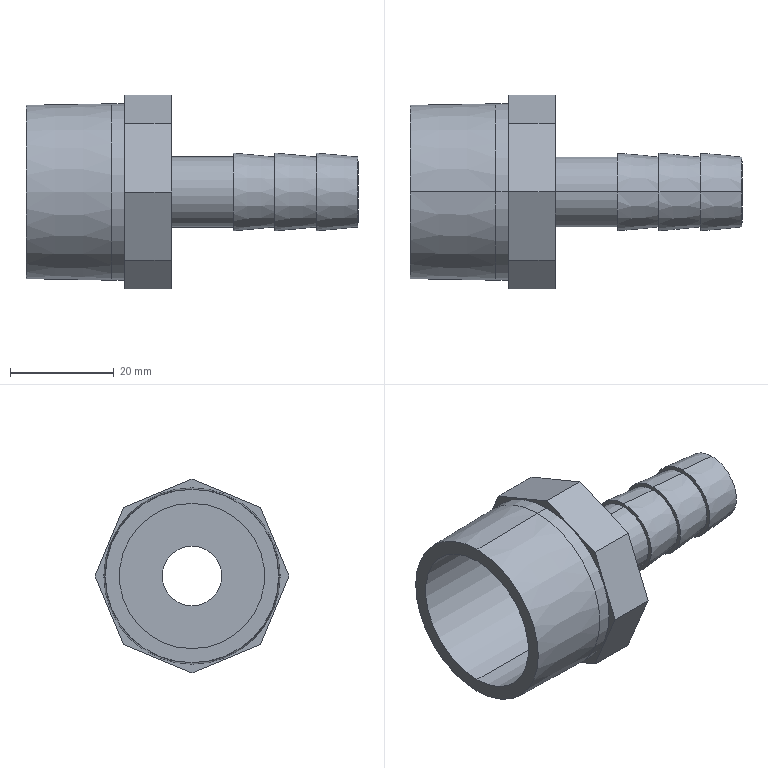Part | SolidWorks | features ICE 1, Revolution 1 | 1 solid | 32 faces | box 64 x 37.343 x 37.343 mm | volume 11465 mm3 | plane 16 | cone 8 | cylinder 8 | commonest cylinder face diameters 11.5 x2 13.5 x2 28 x2 34 x2
STEP:
#1=CARTESIAN_POINT('',(64.,0.,6.75));
#2=VERTEX_POINT('',#1);
#3=CARTESIAN_POINT('',(64.,0.,-6.75));
#4=VERTEX_POINT('',#3);
#5=CARTESIAN_POINT('',(64.,0.,0.));
#6=DIRECTION('',(-1.,0.,0.));
#7=DIRECTION('',(0.,0.,1.));
#8=AXIS2_PLACEMENT_3D('',#5,#6,#7);
#9=CIRCLE('',#8,6.75);
#10=EDGE_CURVE('',#2,#4,#9,.T.);
#11=ORIENTED_EDGE('',*,*,#10,.T.);
#12=CARTESIAN_POINT('',(56.,0.,-7.5));
#13=VERTEX_POINT('',#12);
#14=CARTESIAN_POINT('',(64.,0.,-6.75));
#15=DIRECTION('',(-0.9956,0.,-0.09334));
#16=VECTOR('',#15,1000.);
#17=LINE('',#14,#16);
#18=EDGE_CURVE('',#4,#13,#17,.T.);
#19=ORIENTED_EDGE('',*,*,#18,.T.);
#20=CARTESIAN_POINT('',(56.,0.,7.5));
#21=VERTEX_POINT('',#20);
#22=CARTESIAN_POINT('',(56.,0.,0.));
#23=DIRECTION('',(-1.,0.,0.));
#24=DIRECTION('',(0.,0.,1.));
#25=AXIS2_PLACEMENT_3D('',#22,#23,#24);
#26=CIRCLE('',#25,7.5);
#27=EDGE_CURVE('',#21,#13,#26,.T.);
#28=ORIENTED_EDGE('',*,*,#27,.F.);
#29=CARTESIAN_POINT('',(64.,0.,6.75));
#30=DIRECTION('',(-0.9956,0.,0.09334));
#31=VECTOR('',#30,1000.);
#32=LINE('',#29,#31);
#33=EDGE_CURVE('',#2,#21,#32,.T.);
#34=ORIENTED_EDGE('',*,*,#33,.F.);
#35=EDGE_LOOP('',(#11,#19,#28,#34));
#36=FACE_OUTER_BOUND('',#35,.T.);
#37=CARTESIAN_POINT('',(64.,0.,0.));
#38=DIRECTION('',(-1.,0.,0.));
#39=DIRECTION('',(0.,0.,1.));
#40=AXIS2_PLACEMENT_3D('',#37,#38,#39);
#41=CONICAL_SURFACE('',#40,6.75,0.09348);
#42=ADVANCED_FACE('',(#36),#41,.T.);
#43=CARTESIAN_POINT('',(64.,0.,-5.75));
#44=VERTEX_POINT('',#43);
#45=CARTESIAN_POINT('',(64.,0.,5.75));
#46=VERTEX_POINT('',#45);
#47=CARTESIAN_POINT('',(64.,0.,0.));
#48=DIRECTION('',(-1.,0.,0.));
#49=DIRECTION('',(0.,0.,1.));
#50=AXIS2_PLACEMENT_3D('',#47,#48,#49);
#51=CIRCLE('',#50,5.75);
#52=EDGE_CURVE('',#44,#46,#51,.T.);
#53=ORIENTED_EDGE('',*,*,#52,.F.);
#54=CARTESIAN_POINT('',(26.,0.,-5.75));
#55=VERTEX_POINT('',#54);
#56=CARTESIAN_POINT('',(0.,0.,-5.75));
#57=DIRECTION('',(-1.,0.,0.));
#58=VECTOR('',#57,1000.);
#59=LINE('',#56,#58);
#60=EDGE_CURVE('',#44,#55,#59,.T.);
#61=ORIENTED_EDGE('',*,*,#60,.T.);
#62=CARTESIAN_POINT('',(26.,0.,5.75));
#63=VERTEX_POINT('',#62);
#64=CARTESIAN_POINT('',(26.,0.,0.));
#65=DIRECTION('',(-1.,0.,0.));
#66=DIRECTION('',(0.,0.,1.));
#67=AXIS2_PLACEMENT_3D('',#64,#65,#66);
#68=CIRCLE('',#67,5.75);
#69=EDGE_CURVE('',#55,#63,#68,.T.);
#70=ORIENTED_EDGE('',*,*,#69,.T.);
#71=CARTESIAN_POINT('',(0.,0.,5.75));
#72=DIRECTION('',(-1.,0.,0.));
#73=VECTOR('',#72,1000.);
#74=LINE('',#71,#73);
#75=EDGE_CURVE('',#46,#63,#74,.T.);
#76=ORIENTED_EDGE('',*,*,#75,.F.);
#77=EDGE_LOOP('',(#53,#61,#70,#76));
#78=FACE_OUTER_BOUND('',#77,.T.);
#79=CARTESIAN_POINT('',(0.,0.,0.));
#80=DIRECTION('',(-1.,0.,0.));
#81=DIRECTION('',(0.,0.,1.));
#82=AXIS2_PLACEMENT_3D('',#79,#80,#81);
#83=CYLINDRICAL_SURFACE('',#82,5.75);
#84=ADVANCED_FACE('',(#78),#83,.F.);
#85=CARTESIAN_POINT('',(26.,0.,-14.));
#86=VERTEX_POINT('',#85);
#87=CARTESIAN_POINT('',(26.,0.,14.));
#88=VERTEX_POINT('',#87);
#89=CARTESIAN_POINT('',(26.,0.,0.));
#90=DIRECTION('',(-1.,0.,0.));
#91=DIRECTION('',(0.,0.,1.));
#92=AXIS2_PLACEMENT_3D('',#89,#90,#91);
#93=CIRCLE('',#92,14.);
#94=EDGE_CURVE('',#86,#88,#93,.T.);
#95=ORIENTED_EDGE('',*,*,#94,.F.);
#96=CARTESIAN_POINT('',(0.,0.,-14.));
#97=VERTEX_POINT('',#96);
#98=CARTESIAN_POINT('',(0.,0.,-14.));
#99=DIRECTION('',(-1.,0.,0.));
#100=VECTOR('',#99,1000.);
#101=LINE('',#98,#100);
#102=EDGE_CURVE('',#86,#97,#101,.T.);
#103=ORIENTED_EDGE('',*,*,#102,.T.);
#104=CARTESIAN_POINT('',(0.,0.,14.));
#105=VERTEX_POINT('',#104);
#106=CARTESIAN_POINT('',(0.,0.,0.));
#107=DIRECTION('',(-1.,0.,0.));
#108=DIRECTION('',(0.,0.,1.));
#109=AXIS2_PLACEMENT_3D('',#106,#107,#108);
#110=CIRCLE('',#109,14.);
#111=EDGE_CURVE('',#97,#105,#110,.T.);
#112=ORIENTED_EDGE('',*,*,#111,.T.);
#113=CARTESIAN_POINT('',(0.,0.,14.));
#114=DIRECTION('',(-1.,0.,0.));
#115=VECTOR('',#114,1000.);
#116=LINE('',#113,#115);
#117=EDGE_CURVE('',#88,#105,#116,.T.);
#118=ORIENTED_EDGE('',*,*,#117,.F.);
#119=EDGE_LOOP('',(#95,#103,#112,#118));
#120=FACE_OUTER_BOUND('',#119,.T.);
#121=CARTESIAN_POINT('',(0.,0.,0.));
#122=DIRECTION('',(-1.,0.,0.));
#123=DIRECTION('',(0.,0.,1.));
#124=AXIS2_PLACEMENT_3D('',#121,#122,#123);
#125=CYLINDRICAL_SURFACE('',#124,14.);
#126=ADVANCED_FACE('',(#120),#125,.F.);
#127=CARTESIAN_POINT('',(0.,0.,16.712));
#128=VERTEX_POINT('',#127);
#129=CARTESIAN_POINT('',(0.,0.,-16.712));
#130=VERTEX_POINT('',#129);
#131=CARTESIAN_POINT('',(0.,0.,0.));
#132=DIRECTION('',(-1.,0.,0.));
#133=DIRECTION('',(0.,0.,1.));
#134=AXIS2_PLACEMENT_3D('',#131,#132,#133);
#135=CIRCLE('',#134,16.712);
#136=EDGE_CURVE('',#128,#130,#135,.T.);
#137=ORIENTED_EDGE('',*,*,#136,.F.);
#138=CARTESIAN_POINT('',(16.5,0.,17.));
#139=VERTEX_POINT('',#138);
#140=CARTESIAN_POINT('',(16.5,0.,17.));
#141=DIRECTION('',(0.9998,0.,0.01745));
#142=VECTOR('',#141,1000.);
#143=LINE('',#140,#142);
#144=EDGE_CURVE('',#128,#139,#143,.T.);
#145=ORIENTED_EDGE('',*,*,#144,.T.);
#146=CARTESIAN_POINT('',(16.5,0.,-17.));
#147=VERTEX_POINT('',#146);
#148=CARTESIAN_POINT('',(16.5,0.,0.));
#149=DIRECTION('',(-1.,0.,0.));
#150=DIRECTION('',(0.,0.,1.));
#151=AXIS2_PLACEMENT_3D('',#148,#149,#150);
#152=CIRCLE('',#151,17.);
#153=EDGE_CURVE('',#139,#147,#152,.T.);
#154=ORIENTED_EDGE('',*,*,#153,.T.);
#155=CARTESIAN_POINT('',(16.5,0.,-17.));
#156=DIRECTION('',(0.9998,0.,-0.01745));
#157=VECTOR('',#156,1000.);
#158=LINE('',#155,#157);
#159=EDGE_CURVE('',#130,#147,#158,.T.);
#160=ORIENTED_EDGE('',*,*,#159,.F.);
#161=EDGE_LOOP('',(#137,#145,#154,#160));
#162=FACE_OUTER_BOUND('',#161,.T.);
#163=CARTESIAN_POINT('',(16.5,0.,0.));
#164=DIRECTION('',(1.,0.,0.));
#165=DIRECTION('',(0.,0.,-1.));
#166=AXIS2_PLACEMENT_3D('',#163,#164,#165);
#167=CONICAL_SURFACE('',#166,17.,0.01745);
#168=ADVANCED_FACE('',(#162),#167,.T.);
#169=CARTESIAN_POINT('',(19.,0.,17.));
#170=VERTEX_POINT('',#169);
#171=CARTESIAN_POINT('',(19.,0.,-17.));
#172=VERTEX_POINT('',#171);
#173=CARTESIAN_POINT('',(19.,0.,0.));
#174=DIRECTION('',(-1.,0.,0.));
#175=DIRECTION('',(0.,0.,1.));
#176=AXIS2_PLACEMENT_3D('',#173,#174,#175);
#177=CIRCLE('',#176,17.);
#178=EDGE_CURVE('',#170,#172,#177,.T.);
#179=ORIENTED_EDGE('',*,*,#178,.T.);
#180=CARTESIAN_POINT('',(0.,0.,-17.));
#181=DIRECTION('',(-1.,0.,0.));
#182=VECTOR('',#181,1000.);
#183=LINE('',#180,#182);
#184=EDGE_CURVE('',#172,#147,#183,.T.);
#185=ORIENTED_EDGE('',*,*,#184,.T.);
#186=ORIENTED_EDGE('',*,*,#153,.F.);
#187=CARTESIAN_POINT('',(0.,0.,17.));
#188=DIRECTION('',(-1.,0.,0.));
#189=VECTOR('',#188,1000.);
#190=LINE('',#187,#189);
#191=EDGE_CURVE('',#170,#139,#190,.T.);
#192=ORIENTED_EDGE('',*,*,#191,.F.);
#193=EDGE_LOOP('',(#179,#185,#186,#192));
#194=FACE_OUTER_BOUND('',#193,.T.);
#195=CARTESIAN_POINT('',(0.,0.,0.));
#196=DIRECTION('',(-1.,0.,0.));
#197=DIRECTION('',(0.,0.,1.));
#198=AXIS2_PLACEMENT_3D('',#195,#196,#197);
#199=CYLINDRICAL_SURFACE('',#198,17.);
#200=ADVANCED_FACE('',(#194),#199,.T.);
#201=CARTESIAN_POINT('',(40.,0.,6.75));
#202=VERTEX_POINT('',#201);
#203=CARTESIAN_POINT('',(40.,0.,-6.75));
#204=VERTEX_POINT('',#203);
#205=CARTESIAN_POINT('',(40.,0.,0.));
#206=DIRECTION('',(-1.,0.,0.));
#207=DIRECTION('',(0.,0.,1.));
#208=AXIS2_PLACEMENT_3D('',#205,#206,#207);
#209=CIRCLE('',#208,6.75);
#210=EDGE_CURVE('',#202,#204,#209,.T.);
#211=ORIENTED_EDGE('',*,*,#210,.T.);
#212=CARTESIAN_POINT('',(28.,0.,-6.75));
#213=VERTEX_POINT('',#212);
#214=CARTESIAN_POINT('',(0.,0.,-6.75));
#215=DIRECTION('',(-1.,0.,0.));
#216=VECTOR('',#215,1000.);
#217=LINE('',#214,#216);
#218=EDGE_CURVE('',#204,#213,#217,.T.);
#219=ORIENTED_EDGE('',*,*,#218,.T.);
#220=CARTESIAN_POINT('',(28.,0.,6.75));
#221=VERTEX_POINT('',#220);
#222=CARTESIAN_POINT('',(28.,0.,0.));
#223=DIRECTION('',(-1.,0.,0.));
#224=DIRECTION('',(0.,0.,1.));
#225=AXIS2_PLACEMENT_3D('',#222,#223,#224);
#226=CIRCLE('',#225,6.75);
#227=EDGE_CURVE('',#221,#213,#226,.T.);
#228=ORIENTED_EDGE('',*,*,#227,.F.);
#229=CARTESIAN_POINT('',(0.,0.,6.75));
#230=DIRECTION('',(-1.,0.,0.));
#231=VECTOR('',#230,1000.);
#232=LINE('',#229,#231);
#233=EDGE_CURVE('',#202,#221,#232,.T.);
#234=ORIENTED_EDGE('',*,*,#233,.F.);
#235=EDGE_LOOP('',(#211,#219,#228,#234));
#236=FACE_OUTER_BOUND('',#235,.T.);
#237=CARTESIAN_POINT('',(0.,0.,0.));
#238=DIRECTION('',(-1.,0.,0.));
#239=DIRECTION('',(0.,0.,1.));
#240=AXIS2_PLACEMENT_3D('',#237,#238,#239);
#241=CYLINDRICAL_SURFACE('',#240,6.75);
#242=ADVANCED_FACE('',(#236),#241,.T.);
#243=CARTESIAN_POINT('',(48.,0.,6.75));
#244=VERTEX_POINT('',#243);
#245=CARTESIAN_POINT('',(48.,0.,-6.75));
#246=VERTEX_POINT('',#245);
#247=CARTESIAN_POINT('',(48.,0.,0.));
#248=DIRECTION('',(-1.,0.,0.));
#249=DIRECTION('',(0.,0.,1.));
#250=AXIS2_PLACEMENT_3D('',#247,#248,#249);
#251=CIRCLE('',#250,6.75);
#252=EDGE_CURVE('',#244,#246,#251,.T.);
#253=ORIENTED_EDGE('',*,*,#252,.T.);
#254=CARTESIAN_POINT('',(40.,0.,-7.5));
#255=VERTEX_POINT('',#254);
#256=CARTESIAN_POINT('',(48.,0.,-6.75));
#257=DIRECTION('',(-0.9956,0.,-0.09334));
#258=VECTOR('',#257,1000.);
#259=LINE('',#256,#258);
#260=EDGE_CURVE('',#246,#255,#259,.T.);
#261=ORIENTED_EDGE('',*,*,#260,.T.);
#262=CARTESIAN_POINT('',(40.,0.,7.5));
#263=VERTEX_POINT('',#262);
#264=CARTESIAN_POINT('',(40.,0.,0.));
#265=DIRECTION('',(-1.,0.,0.));
#266=DIRECTION('',(0.,0.,1.));
#267=AXIS2_PLACEMENT_3D('',#264,#265,#266);
#268=CIRCLE('',#267,7.5);
#269=EDGE_CURVE('',#263,#255,#268,.T.);
#270=ORIENTED_EDGE('',*,*,#269,.F.);
#271=CARTESIAN_POINT('',(48.,0.,6.75));
#272=DIRECTION('',(-0.9956,0.,0.09334));
#273=VECTOR('',#272,1000.);
#274=LINE('',#271,#273);
#275=EDGE_CURVE('',#244,#263,#274,.T.);
#276=ORIENTED_EDGE('',*,*,#275,.F.);
#277=EDGE_LOOP('',(#253,#261,#270,#276));
#278=FACE_OUTER_BOUND('',#277,.T.);
#279=CARTESIAN_POINT('',(48.,0.,0.));
#280=DIRECTION('',(-1.,0.,0.));
#281=DIRECTION('',(0.,0.,1.));
#282=AXIS2_PLACEMENT_3D('',#279,#280,#281);
#283=CONICAL_SURFACE('',#282,6.75,0.09348);
#284=ADVANCED_FACE('',(#278),#283,.T.);
#285=CARTESIAN_POINT('',(56.,0.,6.75));
#286=VERTEX_POINT('',#285);
#287=CARTESIAN_POINT('',(56.,0.,-6.75));
#288=VERTEX_POINT('',#287);
#289=CARTESIAN_POINT('',(56.,0.,0.));
#290=DIRECTION('',(-1.,0.,0.));
#291=DIRECTION('',(0.,0.,1.));
#292=AXIS2_PLACEMENT_3D('',#289,#290,#291);
#293=CIRCLE('',#292,6.75);
#294=EDGE_CURVE('',#286,#288,#293,.T.);
#295=ORIENTED_EDGE('',*,*,#294,.T.);
#296=CARTESIAN_POINT('',(48.,0.,-7.5));
#297=VERTEX_POINT('',#296);
#298=CARTESIAN_POINT('',(56.,0.,-6.75));
#299=DIRECTION('',(-0.9956,0.,-0.09334));
#300=VECTOR('',#299,1000.);
#301=LINE('',#298,#300);
#302=EDGE_CURVE('',#288,#297,#301,.T.);
#303=ORIENTED_EDGE('',*,*,#302,.T.);
#304=CARTESIAN_POINT('',(48.,0.,7.5));
#305=VERTEX_POINT('',#304);
#306=CARTESIAN_POINT('',(48.,0.,0.));
#307=DIRECTION('',(-1.,0.,0.));
#308=DIRECTION('',(0.,0.,1.));
#309=AXIS2_PLACEMENT_3D('',#306,#307,#308);
#310=CIRCLE('',#309,7.5);
#311=EDGE_CURVE('',#305,#297,#310,.T.);
#312=ORIENTED_EDGE('',*,*,#311,.F.);
#313=CARTESIAN_POINT('',(56.,0.,6.75));
#314=DIRECTION('',(-0.9956,0.,0.09334));
#315=VECTOR('',#314,1000.);
#316=LINE('',#313,#315);
#317=EDGE_CURVE('',#286,#305,#316,.T.);
#318=ORIENTED_EDGE('',*,*,#317,.F.);
#319=EDGE_LOOP('',(#295,#303,#312,#318));
#320=FACE_OUTER_BOUND('',#319,.T.);
#321=CARTESIAN_POINT('',(56.,0.,0.));
#322=DIRECTION('',(-1.,0.,0.));
#323=DIRECTION('',(0.,0.,1.));
#324=AXIS2_PLACEMENT_3D('',#321,#322,#323);
#325=CONICAL_SURFACE('',#324,6.75,0.09348);
#326=ADVANCED_FACE('',(#320),#325,.T.);
#327=ORIENTED_EDGE('',*,*,#302,.F.);
#328=CARTESIAN_POINT('',(56.,0.,0.));
#329=DIRECTION('',(-1.,0.,0.));
#330=DIRECTION('',(0.,0.,1.));
#331=AXIS2_PLACEMENT_3D('',#328,#329,#330);
#332=CIRCLE('',#331,6.75);
#333=EDGE_CURVE('',#288,#286,#332,.T.);
#334=ORIENTED_EDGE('',*,*,#333,.T.);
#335=ORIENTED_EDGE('',*,*,#317,.T.);
#336=CARTESIAN_POINT('',(48.,0.,0.));
#337=DIRECTION('',(-1.,0.,0.));
#338=DIRECTION('',(0.,0.,1.));
#339=AXIS2_PLACEMENT_3D('',#336,#337,#338);
#340=CIRCLE('',#339,7.5);
#341=EDGE_CURVE('',#297,#305,#340,.T.);
#342=ORIENTED_EDGE('',*,*,#341,.F.);
#343=EDGE_LOOP('',(#327,#334,#335,#342));
#344=FACE_OUTER_BOUND('',#343,.T.);
#345=CARTESIAN_POINT('',(56.,0.,0.));
#346=DIRECTION('',(-1.,0.,0.));
#347=DIRECTION('',(0.,0.,1.));
#348=AXIS2_PLACEMENT_3D('',#345,#346,#347);
#349=CONICAL_SURFACE('',#348,6.75,0.09348);
#350=ADVANCED_FACE('',(#344),#349,.T.);
#351=ORIENTED_EDGE('',*,*,#252,.F.);
#352=CARTESIAN_POINT('',(48.,0.,0.));
#353=DIRECTION('',(-1.,0.,0.));
#354=DIRECTION('',(0.,0.,1.));
#355=AXIS2_PLACEMENT_3D('',#352,#353,#354);
#356=CIRCLE('',#355,6.75);
#357=EDGE_CURVE('',#246,#244,#356,.T.);
#358=ORIENTED_EDGE('',*,*,#357,.F.);
#359=EDGE_LOOP('',(#351,#358));
#360=FACE_BOUND('',#359,.T.);
#361=ORIENTED_EDGE('',*,*,#311,.T.);
#362=ORIENTED_EDGE('',*,*,#341,.T.);
#363=EDGE_LOOP('',(#361,#362));
#364=FACE_OUTER_BOUND('',#363,.T.);
#365=CARTESIAN_POINT('',(48.,7.5,0.));
#366=DIRECTION('',(1.,0.,0.));
#367=DIRECTION('',(0.,0.,-1.));
#368=AXIS2_PLACEMENT_3D('',#365,#366,#367);
#369=PLANE('',#368);
#370=ADVANCED_FACE('',(#360,#364),#369,.F.);
#371=ORIENTED_EDGE('',*,*,#260,.F.);
#372=ORIENTED_EDGE('',*,*,#357,.T.);
#373=ORIENTED_EDGE('',*,*,#275,.T.);
#374=CARTESIAN_POINT('',(40.,0.,0.));
#375=DIRECTION('',(-1.,0.,0.));
#376=DIRECTION('',(0.,0.,1.));
#377=AXIS2_PLACEMENT_3D('',#374,#375,#376);
#378=CIRCLE('',#377,7.5);
#379=EDGE_CURVE('',#255,#263,#378,.T.);
#380=ORIENTED_EDGE('',*,*,#379,.F.);
#381=EDGE_LOOP('',(#371,#372,#373,#380));
#382=FACE_OUTER_BOUND('',#381,.T.);
#383=CARTESIAN_POINT('',(48.,0.,0.));
#384=DIRECTION('',(-1.,0.,0.));
#385=DIRECTION('',(0.,0.,1.));
#386=AXIS2_PLACEMENT_3D('',#383,#384,#385);
#387=CONICAL_SURFACE('',#386,6.75,0.09348);
#388=ADVANCED_FACE('',(#382),#387,.T.);
#389=ORIENTED_EDGE('',*,*,#210,.F.);
#390=CARTESIAN_POINT('',(40.,0.,0.));
#391=DIRECTION('',(-1.,0.,0.));
#392=DIRECTION('',(0.,0.,1.));
#393=AXIS2_PLACEMENT_3D('',#390,#391,#392);
#394=CIRCLE('',#393,6.75);
#395=EDGE_CURVE('',#204,#202,#394,.T.);
#396=ORIENTED_EDGE('',*,*,#395,.F.);
#397=EDGE_LOOP('',(#389,#396));
#398=FACE_BOUND('',#397,.T.);
#399=ORIENTED_EDGE('',*,*,#269,.T.);
#400=ORIENTED_EDGE('',*,*,#379,.T.);
#401=EDGE_LOOP('',(#399,#400));
#402=FACE_OUTER_BOUND('',#401,.T.);
#403=CARTESIAN_POINT('',(40.,7.5,0.));
#404=DIRECTION('',(1.,0.,0.));
#405=DIRECTION('',(0.,0.,-1.));
#406=AXIS2_PLACEMENT_3D('',#403,#404,#405);
#407=PLANE('',#406);
#408=ADVANCED_FACE('',(#398,#402),#407,.F.);
#409=ORIENTED_EDGE('',*,*,#218,.F.);
#410=ORIENTED_EDGE('',*,*,#395,.T.);
#411=ORIENTED_EDGE('',*,*,#233,.T.);
#412=CARTESIAN_POINT('',(28.,0.,0.));
#413=DIRECTION('',(-1.,0.,0.));
#414=DIRECTION('',(0.,0.,1.));
#415=AXIS2_PLACEMENT_3D('',#412,#413,#414);
#416=CIRCLE('',#415,6.75);
#417=EDGE_CURVE('',#213,#221,#416,.T.);
#418=ORIENTED_EDGE('',*,*,#417,.F.);
#419=EDGE_LOOP('',(#409,#410,#411,#418));
#420=FACE_OUTER_BOUND('',#419,.T.);
#421=CARTESIAN_POINT('',(0.,0.,0.));
#422=DIRECTION('',(-1.,0.,0.));
#423=DIRECTION('',(0.,0.,1.));
#424=AXIS2_PLACEMENT_3D('',#421,#422,#423);
#425=CYLINDRICAL_SURFACE('',#424,6.75);
#426=ADVANCED_FACE('',(#420),#425,.T.);
#427=CARTESIAN_POINT('',(28.,-13.203,-13.203));
#428=VERTEX_POINT('',#427);
#429=CARTESIAN_POINT('',(28.,0.,-18.671));
#430=VERTEX_POINT('',#429);
#431=CARTESIAN_POINT('',(28.,-13.203,-13.203));
#432=DIRECTION('',(0.,0.9239,-0.3827));
#433=VECTOR('',#432,1000.);
#434=LINE('',#431,#433);
#435=EDGE_CURVE('',#428,#430,#434,.T.);
#436=ORIENTED_EDGE('',*,*,#435,.T.);
#437=CARTESIAN_POINT('',(28.,13.203,-13.203));
#438=VERTEX_POINT('',#437);
#439=CARTESIAN_POINT('',(28.,0.,-18.671));
#440=DIRECTION('',(0.,0.9239,0.3827));
#441=VECTOR('',#440,1000.);
#442=LINE('',#439,#441);
#443=EDGE_CURVE('',#430,#438,#442,.T.);
#444=ORIENTED_EDGE('',*,*,#443,.T.);
#445=CARTESIAN_POINT('',(28.,18.671,0.));
#446=VERTEX_POINT('',#445);
#447=CARTESIAN_POINT('',(28.,13.203,-13.203));
#448=DIRECTION('',(0.,0.3827,0.9239));
#449=VECTOR('',#448,1000.);
#450=LINE('',#447,#449);
#451=EDGE_CURVE('',#438,#446,#450,.T.);
#452=ORIENTED_EDGE('',*,*,#451,.T.);
#453=CARTESIAN_POINT('',(28.,13.203,13.203));
#454=VERTEX_POINT('',#453);
#455=CARTESIAN_POINT('',(28.,18.671,0.));
#456=DIRECTION('',(0.,-0.3827,0.9239));
#457=VECTOR('',#456,1000.);
#458=LINE('',#455,#457);
#459=EDGE_CURVE('',#446,#454,#458,.T.);
#460=ORIENTED_EDGE('',*,*,#459,.T.);
#461=CARTESIAN_POINT('',(28.,0.,18.671));
#462=VERTEX_POINT('',#461);
#463=CARTESIAN_POINT('',(28.,13.203,13.203));
#464=DIRECTION('',(0.,-0.9239,0.3827));
#465=VECTOR('',#464,1000.);
#466=LINE('',#463,#465);
#467=EDGE_CURVE('',#454,#462,#466,.T.);
#468=ORIENTED_EDGE('',*,*,#467,.T.);
#469=CARTESIAN_POINT('',(28.,-13.203,13.203));
#470=VERTEX_POINT('',#469);
#471=CARTESIAN_POINT('',(28.,0.,18.671));
#472=DIRECTION('',(0.,-0.9239,-0.3827));
#473=VECTOR('',#472,1000.);
#474=LINE('',#471,#473);
#475=EDGE_CURVE('',#462,#470,#474,.T.);
#476=ORIENTED_EDGE('',*,*,#475,.T.);
#477=CARTESIAN_POINT('',(28.,-18.671,0.));
#478=VERTEX_POINT('',#477);
#479=CARTESIAN_POINT('',(28.,-13.203,13.203));
#480=DIRECTION('',(0.,-0.3827,-0.9239));
#481=VECTOR('',#480,1000.);
#482=LINE('',#479,#481);
#483=EDGE_CURVE('',#470,#478,#482,.T.);
#484=ORIENTED_EDGE('',*,*,#483,.T.);
#485=CARTESIAN_POINT('',(28.,-18.671,0.));
#486=DIRECTION('',(0.,0.3827,-0.9239));
#487=VECTOR('',#486,1000.);
#488=LINE('',#485,#487);
#489=EDGE_CURVE('',#478,#428,#488,.T.);
#490=ORIENTED_EDGE('',*,*,#489,.T.);
#491=EDGE_LOOP('',(#436,#444,#452,#460,#468,#476,#484,#490));
#492=FACE_OUTER_BOUND('',#491,.T.);
#493=ORIENTED_EDGE('',*,*,#227,.T.);
#494=ORIENTED_EDGE('',*,*,#417,.T.);
#495=EDGE_LOOP('',(#493,#494));
#496=FACE_BOUND('',#495,.T.);
#497=CARTESIAN_POINT('',(28.,17.25,0.));
#498=DIRECTION('',(-1.,0.,0.));
#499=DIRECTION('',(0.,0.,1.));
#500=AXIS2_PLACEMENT_3D('',#497,#498,#499);
#501=PLANE('',#500);
#502=ADVANCED_FACE('',(#492,#496),#501,.F.);
#503=ORIENTED_EDGE('',*,*,#178,.F.);
#504=CARTESIAN_POINT('',(19.,0.,0.));
#505=DIRECTION('',(-1.,0.,0.));
#506=DIRECTION('',(0.,0.,1.));
#507=AXIS2_PLACEMENT_3D('',#504,#505,#506);
#508=CIRCLE('',#507,17.);
#509=EDGE_CURVE('',#172,#170,#508,.T.);
#510=ORIENTED_EDGE('',*,*,#509,.F.);
#511=EDGE_LOOP('',(#503,#510));
#512=FACE_BOUND('',#511,.T.);
#513=CARTESIAN_POINT('',(19.,-13.203,13.203));
#514=VERTEX_POINT('',#513);
#515=CARTESIAN_POINT('',(19.,0.,18.671));
#516=VERTEX_POINT('',#515);
#517=CARTESIAN_POINT('',(19.,0.,18.671));
#518=DIRECTION('',(0.,0.9239,0.3827));
#519=VECTOR('',#518,1000.);
#520=LINE('',#517,#519);
#521=EDGE_CURVE('',#514,#516,#520,.T.);
#522=ORIENTED_EDGE('',*,*,#521,.T.);
#523=CARTESIAN_POINT('',(19.,13.203,13.203));
#524=VERTEX_POINT('',#523);
#525=CARTESIAN_POINT('',(19.,13.203,13.203));
#526=DIRECTION('',(0.,0.9239,-0.3827));
#527=VECTOR('',#526,1000.);
#528=LINE('',#525,#527);
#529=EDGE_CURVE('',#516,#524,#528,.T.);
#530=ORIENTED_EDGE('',*,*,#529,.T.);
#531=CARTESIAN_POINT('',(19.,18.671,0.));
#532=VERTEX_POINT('',#531);
#533=CARTESIAN_POINT('',(19.,18.671,0.));
#534=DIRECTION('',(0.,0.3827,-0.9239));
#535=VECTOR('',#534,1000.);
#536=LINE('',#533,#535);
#537=EDGE_CURVE('',#524,#532,#536,.T.);
#538=ORIENTED_EDGE('',*,*,#537,.T.);
#539=CARTESIAN_POINT('',(19.,13.203,-13.203));
#540=VERTEX_POINT('',#539);
#541=CARTESIAN_POINT('',(19.,13.203,-13.203));
#542=DIRECTION('',(0.,-0.3827,-0.9239));
#543=VECTOR('',#542,1000.);
#544=LINE('',#541,#543);
#545=EDGE_CURVE('',#532,#540,#544,.T.);
#546=ORIENTED_EDGE('',*,*,#545,.T.);
#547=CARTESIAN_POINT('',(19.,0.,-18.671));
#548=VERTEX_POINT('',#547);
#549=CARTESIAN_POINT('',(19.,0.,-18.671));
#550=DIRECTION('',(0.,-0.9239,-0.3827));
#551=VECTOR('',#550,1000.);
#552=LINE('',#549,#551);
#553=EDGE_CURVE('',#540,#548,#552,.T.);
#554=ORIENTED_EDGE('',*,*,#553,.T.);
#555=CARTESIAN_POINT('',(19.,-13.203,-13.203));
#556=VERTEX_POINT('',#555);
#557=CARTESIAN_POINT('',(19.,-13.203,-13.203));
#558=DIRECTION('',(0.,-0.9239,0.3827));
#559=VECTOR('',#558,1000.);
#560=LINE('',#557,#559);
#561=EDGE_CURVE('',#548,#556,#560,.T.);
#562=ORIENTED_EDGE('',*,*,#561,.T.);
#563=CARTESIAN_POINT('',(19.,-18.671,0.));
#564=VERTEX_POINT('',#563);
#565=CARTESIAN_POINT('',(19.,-18.671,0.));
#566=DIRECTION('',(0.,-0.3827,0.9239));
#567=VECTOR('',#566,1000.);
#568=LINE('',#565,#567);
#569=EDGE_CURVE('',#556,#564,#568,.T.);
#570=ORIENTED_EDGE('',*,*,#569,.T.);
#571=CARTESIAN_POINT('',(19.,-13.203,13.203));
#572=DIRECTION('',(0.,0.3827,0.9239));
#573=VECTOR('',#572,1000.);
#574=LINE('',#571,#573);
#575=EDGE_CURVE('',#564,#514,#574,.T.);
#576=ORIENTED_EDGE('',*,*,#575,.T.);
#577=EDGE_LOOP('',(#522,#530,#538,#546,#554,#562,#570,#576));
#578=FACE_OUTER_BOUND('',#577,.T.);
#579=CARTESIAN_POINT('',(19.,17.,0.));
#580=DIRECTION('',(1.,0.,0.));
#581=DIRECTION('',(0.,0.,-1.));
#582=AXIS2_PLACEMENT_3D('',#579,#580,#581);
#583=PLANE('',#582);
#584=ADVANCED_FACE('',(#512,#578),#583,.F.);
#585=ORIENTED_EDGE('',*,*,#184,.F.);
#586=ORIENTED_EDGE('',*,*,#509,.T.);
#587=ORIENTED_EDGE('',*,*,#191,.T.);
#588=CARTESIAN_POINT('',(16.5,0.,0.));
#589=DIRECTION('',(-1.,0.,0.));
#590=DIRECTION('',(0.,0.,1.));
#591=AXIS2_PLACEMENT_3D('',#588,#589,#590);
#592=CIRCLE('',#591,17.);
#593=EDGE_CURVE('',#147,#139,#592,.T.);
#594=ORIENTED_EDGE('',*,*,#593,.F.);
#595=EDGE_LOOP('',(#585,#586,#587,#594));
#596=FACE_OUTER_BOUND('',#595,.T.);
#597=CARTESIAN_POINT('',(0.,0.,0.));
#598=DIRECTION('',(-1.,0.,0.));
#599=DIRECTION('',(0.,0.,1.));
#600=AXIS2_PLACEMENT_3D('',#597,#598,#599);
#601=CYLINDRICAL_SURFACE('',#600,17.);
#602=ADVANCED_FACE('',(#596),#601,.T.);
#603=ORIENTED_EDGE('',*,*,#144,.F.);
#604=CARTESIAN_POINT('',(0.,0.,0.));
#605=DIRECTION('',(-1.,0.,0.));
#606=DIRECTION('',(0.,0.,1.));
#607=AXIS2_PLACEMENT_3D('',#604,#605,#606);
#608=CIRCLE('',#607,16.712);
#609=EDGE_CURVE('',#130,#128,#608,.T.);
#610=ORIENTED_EDGE('',*,*,#609,.F.);
#611=ORIENTED_EDGE('',*,*,#159,.T.);
#612=ORIENTED_EDGE('',*,*,#593,.T.);
#613=EDGE_LOOP('',(#603,#610,#611,#612));
#614=FACE_OUTER_BOUND('',#613,.T.);
#615=CARTESIAN_POINT('',(16.5,0.,0.));
#616=DIRECTION('',(1.,0.,0.));
#617=DIRECTION('',(0.,0.,-1.));
#618=AXIS2_PLACEMENT_3D('',#615,#616,#617);
#619=CONICAL_SURFACE('',#618,17.,0.01745);
#620=ADVANCED_FACE('',(#614),#619,.T.);
#621=CARTESIAN_POINT('',(0.,0.,0.));
#622=DIRECTION('',(-1.,0.,0.));
#623=DIRECTION('',(0.,0.,1.));
#624=AXIS2_PLACEMENT_3D('',#621,#622,#623);
#625=CIRCLE('',#624,14.);
#626=EDGE_CURVE('',#105,#97,#625,.T.);
#627=ORIENTED_EDGE('',*,*,#626,.F.);
#628=ORIENTED_EDGE('',*,*,#111,.F.);
#629=EDGE_LOOP('',(#627,#628));
#630=FACE_BOUND('',#629,.T.);
#631=ORIENTED_EDGE('',*,*,#609,.T.);
#632=ORIENTED_EDGE('',*,*,#136,.T.);
#633=EDGE_LOOP('',(#631,#632));
#634=FACE_OUTER_BOUND('',#633,.T.);
#635=CARTESIAN_POINT('',(0.,16.712,0.));
#636=DIRECTION('',(1.,0.,0.));
#637=DIRECTION('',(0.,0.,-1.));
#638=AXIS2_PLACEMENT_3D('',#635,#636,#637);
#639=PLANE('',#638);
#640=ADVANCED_FACE('',(#630,#634),#639,.F.);
#641=ORIENTED_EDGE('',*,*,#102,.F.);
#642=CARTESIAN_POINT('',(26.,0.,0.));
#643=DIRECTION('',(-1.,0.,0.));
#644=DIRECTION('',(0.,0.,1.));
#645=AXIS2_PLACEMENT_3D('',#642,#643,#644);
#646=CIRCLE('',#645,14.);
#647=EDGE_CURVE('',#88,#86,#646,.T.);
#648=ORIENTED_EDGE('',*,*,#647,.F.);
#649=ORIENTED_EDGE('',*,*,#117,.T.);
#650=ORIENTED_EDGE('',*,*,#626,.T.);
#651=EDGE_LOOP('',(#641,#648,#649,#650));
#652=FACE_OUTER_BOUND('',#651,.T.);
#653=CARTESIAN_POINT('',(0.,0.,0.));
#654=DIRECTION('',(-1.,0.,0.));
#655=DIRECTION('',(0.,0.,1.));
#656=AXIS2_PLACEMENT_3D('',#653,#654,#655);
#657=CYLINDRICAL_SURFACE('',#656,14.);
#658=ADVANCED_FACE('',(#652),#657,.F.);
#659=CARTESIAN_POINT('',(26.,0.,0.));
#660=DIRECTION('',(-1.,0.,0.));
#661=DIRECTION('',(0.,0.,1.));
#662=AXIS2_PLACEMENT_3D('',#659,#660,#661);
#663=CIRCLE('',#662,5.75);
#664=EDGE_CURVE('',#63,#55,#663,.T.);
#665=ORIENTED_EDGE('',*,*,#664,.F.);
#666=ORIENTED_EDGE('',*,*,#69,.F.);
#667=EDGE_LOOP('',(#665,#666));
#668=FACE_BOUND('',#667,.T.);
#669=ORIENTED_EDGE('',*,*,#647,.T.);
#670=ORIENTED_EDGE('',*,*,#94,.T.);
#671=EDGE_LOOP('',(#669,#670));
#672=FACE_OUTER_BOUND('',#671,.T.);
#673=CARTESIAN_POINT('',(26.,5.75,0.));
#674=DIRECTION('',(1.,0.,0.));
#675=DIRECTION('',(0.,0.,-1.));
#676=AXIS2_PLACEMENT_3D('',#673,#674,#675);
#677=PLANE('',#676);
#678=ADVANCED_FACE('',(#668,#672),#677,.F.);
#679=ORIENTED_EDGE('',*,*,#60,.F.);
#680=CARTESIAN_POINT('',(64.,0.,0.));
#681=DIRECTION('',(-1.,0.,0.));
#682=DIRECTION('',(0.,0.,1.));
#683=AXIS2_PLACEMENT_3D('',#680,#681,#682);
#684=CIRCLE('',#683,5.75);
#685=EDGE_CURVE('',#46,#44,#684,.T.);
#686=ORIENTED_EDGE('',*,*,#685,.F.);
#687=ORIENTED_EDGE('',*,*,#75,.T.);
#688=ORIENTED_EDGE('',*,*,#664,.T.);
#689=EDGE_LOOP('',(#679,#686,#687,#688));
#690=FACE_OUTER_BOUND('',#689,.T.);
#691=CARTESIAN_POINT('',(0.,0.,0.));
#692=DIRECTION('',(-1.,0.,0.));
#693=DIRECTION('',(0.,0.,1.));
#694=AXIS2_PLACEMENT_3D('',#691,#692,#693);
#695=CYLINDRICAL_SURFACE('',#694,5.75);
#696=ADVANCED_FACE('',(#690),#695,.F.);
#697=ORIENTED_EDGE('',*,*,#10,.F.);
#698=CARTESIAN_POINT('',(64.,0.,0.));
#699=DIRECTION('',(-1.,0.,0.));
#700=DIRECTION('',(0.,0.,1.));
#701=AXIS2_PLACEMENT_3D('',#698,#699,#700);
#702=CIRCLE('',#701,6.75);
#703=EDGE_CURVE('',#4,#2,#702,.T.);
#704=ORIENTED_EDGE('',*,*,#703,.F.);
#705=EDGE_LOOP('',(#697,#704));
#706=FACE_OUTER_BOUND('',#705,.T.);
#707=ORIENTED_EDGE('',*,*,#685,.T.);
#708=ORIENTED_EDGE('',*,*,#52,.T.);
#709=EDGE_LOOP('',(#707,#708));
#710=FACE_BOUND('',#709,.T.);
#711=CARTESIAN_POINT('',(64.,6.75,0.));
#712=DIRECTION('',(-1.,0.,0.));
#713=DIRECTION('',(0.,0.,1.));
#714=AXIS2_PLACEMENT_3D('',#711,#712,#713);
#715=PLANE('',#714);
#716=ADVANCED_FACE('',(#706,#710),#715,.F.);
#717=ORIENTED_EDGE('',*,*,#18,.F.);
#718=ORIENTED_EDGE('',*,*,#703,.T.);
#719=ORIENTED_EDGE('',*,*,#33,.T.);
#720=CARTESIAN_POINT('',(56.,0.,0.));
#721=DIRECTION('',(-1.,0.,0.));
#722=DIRECTION('',(0.,0.,1.));
#723=AXIS2_PLACEMENT_3D('',#720,#721,#722);
#724=CIRCLE('',#723,7.5);
#725=EDGE_CURVE('',#13,#21,#724,.T.);
#726=ORIENTED_EDGE('',*,*,#725,.F.);
#727=EDGE_LOOP('',(#717,#718,#719,#726));
#728=FACE_OUTER_BOUND('',#727,.T.);
#729=CARTESIAN_POINT('',(64.,0.,0.));
#730=DIRECTION('',(-1.,0.,0.));
#731=DIRECTION('',(0.,0.,1.));
#732=AXIS2_PLACEMENT_3D('',#729,#730,#731);
#733=CONICAL_SURFACE('',#732,6.75,0.09348);
#734=ADVANCED_FACE('',(#728),#733,.T.);
#735=ORIENTED_EDGE('',*,*,#294,.F.);
#736=ORIENTED_EDGE('',*,*,#333,.F.);
#737=EDGE_LOOP('',(#735,#736));
#738=FACE_BOUND('',#737,.T.);
#739=ORIENTED_EDGE('',*,*,#27,.T.);
#740=ORIENTED_EDGE('',*,*,#725,.T.);
#741=EDGE_LOOP('',(#739,#740));
#742=FACE_OUTER_BOUND('',#741,.T.);
#743=CARTESIAN_POINT('',(56.,7.5,0.));
#744=DIRECTION('',(1.,0.,0.));
#745=DIRECTION('',(0.,0.,-1.));
#746=AXIS2_PLACEMENT_3D('',#743,#744,#745);
#747=PLANE('',#746);
#748=ADVANCED_FACE('',(#738,#742),#747,.F.);
#749=ORIENTED_EDGE('',*,*,#537,.F.);
#750=CARTESIAN_POINT('',(-33.81,13.203,13.203));
#751=DIRECTION('',(1.,0.,0.));
#752=VECTOR('',#751,1000.);
#753=LINE('',#750,#752);
#754=EDGE_CURVE('',#524,#454,#753,.T.);
#755=ORIENTED_EDGE('',*,*,#754,.T.);
#756=ORIENTED_EDGE('',*,*,#459,.F.);
#757=CARTESIAN_POINT('',(-33.81,18.671,0.));
#758=DIRECTION('',(1.,0.,0.));
#759=VECTOR('',#758,1000.);
#760=LINE('',#757,#759);
#761=EDGE_CURVE('',#532,#446,#760,.T.);
#762=ORIENTED_EDGE('',*,*,#761,.F.);
#763=EDGE_LOOP('',(#749,#755,#756,#762));
#764=FACE_OUTER_BOUND('',#763,.T.);
#765=CARTESIAN_POINT('',(-33.81,18.671,0.));
#766=DIRECTION('',(0.,0.9239,0.3827));
#767=DIRECTION('',(0.,-0.3827,0.9239));
#768=AXIS2_PLACEMENT_3D('',#765,#766,#767);
#769=PLANE('',#768);
#770=ADVANCED_FACE('',(#764),#769,.T.);
#771=ORIENTED_EDGE('',*,*,#529,.F.);
#772=CARTESIAN_POINT('',(-33.81,0.,18.671));
#773=DIRECTION('',(1.,0.,0.));
#774=VECTOR('',#773,1000.);
#775=LINE('',#772,#774);
#776=EDGE_CURVE('',#516,#462,#775,.T.);
#777=ORIENTED_EDGE('',*,*,#776,.T.);
#778=ORIENTED_EDGE('',*,*,#467,.F.);
#779=ORIENTED_EDGE('',*,*,#754,.F.);
#780=EDGE_LOOP('',(#771,#777,#778,#779));
#781=FACE_OUTER_BOUND('',#780,.T.);
#782=CARTESIAN_POINT('',(-33.81,13.203,13.203));
#783=DIRECTION('',(0.,0.3827,0.9239));
#784=DIRECTION('',(0.,-0.9239,0.3827));
#785=AXIS2_PLACEMENT_3D('',#782,#783,#784);
#786=PLANE('',#785);
#787=ADVANCED_FACE('',(#781),#786,.T.);
#788=ORIENTED_EDGE('',*,*,#521,.F.);
#789=CARTESIAN_POINT('',(-33.81,-13.203,13.203));
#790=DIRECTION('',(1.,0.,0.));
#791=VECTOR('',#790,1000.);
#792=LINE('',#789,#791);
#793=EDGE_CURVE('',#514,#470,#792,.T.);
#794=ORIENTED_EDGE('',*,*,#793,.T.);
#795=ORIENTED_EDGE('',*,*,#475,.F.);
#796=ORIENTED_EDGE('',*,*,#776,.F.);
#797=EDGE_LOOP('',(#788,#794,#795,#796));
#798=FACE_OUTER_BOUND('',#797,.T.);
#799=CARTESIAN_POINT('',(-33.81,0.,18.671));
#800=DIRECTION('',(0.,-0.3827,0.9239));
#801=DIRECTION('',(0.,-0.9239,-0.3827));
#802=AXIS2_PLACEMENT_3D('',#799,#800,#801);
#803=PLANE('',#802);
#804=ADVANCED_FACE('',(#798),#803,.T.);
#805=ORIENTED_EDGE('',*,*,#575,.F.);
#806=CARTESIAN_POINT('',(-33.81,-18.671,0.));
#807=DIRECTION('',(1.,0.,0.));
#808=VECTOR('',#807,1000.);
#809=LINE('',#806,#808);
#810=EDGE_CURVE('',#564,#478,#809,.T.);
#811=ORIENTED_EDGE('',*,*,#810,.T.);
#812=ORIENTED_EDGE('',*,*,#483,.F.);
#813=ORIENTED_EDGE('',*,*,#793,.F.);
#814=EDGE_LOOP('',(#805,#811,#812,#813));
#815=FACE_OUTER_BOUND('',#814,.T.);
#816=CARTESIAN_POINT('',(-33.81,-13.203,13.203));
#817=DIRECTION('',(0.,-0.9239,0.3827));
#818=DIRECTION('',(0.,-0.3827,-0.9239));
#819=AXIS2_PLACEMENT_3D('',#816,#817,#818);
#820=PLANE('',#819);
#821=ADVANCED_FACE('',(#815),#820,.T.);
#822=ORIENTED_EDGE('',*,*,#569,.F.);
#823=CARTESIAN_POINT('',(-33.81,-13.203,-13.203));
#824=DIRECTION('',(1.,0.,0.));
#825=VECTOR('',#824,1000.);
#826=LINE('',#823,#825);
#827=EDGE_CURVE('',#556,#428,#826,.T.);
#828=ORIENTED_EDGE('',*,*,#827,.T.);
#829=ORIENTED_EDGE('',*,*,#489,.F.);
#830=ORIENTED_EDGE('',*,*,#810,.F.);
#831=EDGE_LOOP('',(#822,#828,#829,#830));
#832=FACE_OUTER_BOUND('',#831,.T.);
#833=CARTESIAN_POINT('',(-33.81,-18.671,0.));
#834=DIRECTION('',(0.,-0.9239,-0.3827));
#835=DIRECTION('',(0.,0.3827,-0.9239));
#836=AXIS2_PLACEMENT_3D('',#833,#834,#835);
#837=PLANE('',#836);
#838=ADVANCED_FACE('',(#832),#837,.T.);
#839=ORIENTED_EDGE('',*,*,#561,.F.);
#840=CARTESIAN_POINT('',(-33.81,0.,-18.671));
#841=DIRECTION('',(1.,0.,0.));
#842=VECTOR('',#841,1000.);
#843=LINE('',#840,#842);
#844=EDGE_CURVE('',#548,#430,#843,.T.);
#845=ORIENTED_EDGE('',*,*,#844,.T.);
#846=ORIENTED_EDGE('',*,*,#435,.F.);
#847=ORIENTED_EDGE('',*,*,#827,.F.);
#848=EDGE_LOOP('',(#839,#845,#846,#847));
#849=FACE_OUTER_BOUND('',#848,.T.);
#850=CARTESIAN_POINT('',(-33.81,-13.203,-13.203));
#851=DIRECTION('',(0.,-0.3827,-0.9239));
#852=DIRECTION('',(0.,0.9239,-0.3827));
#853=AXIS2_PLACEMENT_3D('',#850,#851,#852);
#854=PLANE('',#853);
#855=ADVANCED_FACE('',(#849),#854,.T.);
#856=ORIENTED_EDGE('',*,*,#844,.F.);
#857=ORIENTED_EDGE('',*,*,#553,.F.);
#858=CARTESIAN_POINT('',(-33.81,13.203,-13.203));
#859=DIRECTION('',(1.,0.,0.));
#860=VECTOR('',#859,1000.);
#861=LINE('',#858,#860);
#862=EDGE_CURVE('',#540,#438,#861,.T.);
#863=ORIENTED_EDGE('',*,*,#862,.T.);
#864=ORIENTED_EDGE('',*,*,#443,.F.);
#865=EDGE_LOOP('',(#856,#857,#863,#864));
#866=FACE_OUTER_BOUND('',#865,.T.);
#867=CARTESIAN_POINT('',(-33.81,0.,-18.671));
#868=DIRECTION('',(0.,0.3827,-0.9239));
#869=DIRECTION('',(0.,0.9239,0.3827));
#870=AXIS2_PLACEMENT_3D('',#867,#868,#869);
#871=PLANE('',#870);
#872=ADVANCED_FACE('',(#866),#871,.T.);
#873=ORIENTED_EDGE('',*,*,#545,.F.);
#874=ORIENTED_EDGE('',*,*,#761,.T.);
#875=ORIENTED_EDGE('',*,*,#451,.F.);
#876=ORIENTED_EDGE('',*,*,#862,.F.);
#877=EDGE_LOOP('',(#873,#874,#875,#876));
#878=FACE_OUTER_BOUND('',#877,.T.);
#879=CARTESIAN_POINT('',(-33.81,13.203,-13.203));
#880=DIRECTION('',(0.,0.9239,-0.3827));
#881=DIRECTION('',(0.,0.3827,0.9239));
#882=AXIS2_PLACEMENT_3D('',#879,#880,#881);
#883=PLANE('',#882);
#884=ADVANCED_FACE('',(#878),#883,.T.);
#885=CLOSED_SHELL('',(#42,#84,#126,#168,#200,#242,#284,#326,#350,#370,#388,#408,#426,#502,#584,#602,#620,#640,#658,#678,#696,#716,#734,#748,#770,#787,#804,#821,#838,#855,#872,#884));
#886=MANIFOLD_SOLID_BREP('',#885);
#887=CARTESIAN_POINT('',(0.,0.,0.));
#888=DIRECTION('',(0.,0.,1.));
#889=DIRECTION('',(1.,0.,0.));
#890=AXIS2_PLACEMENT_3D('',#887,#888,#889);
#891=(LENGTH_UNIT()NAMED_UNIT(*)SI_UNIT(.MILLI.,.METRE.));
#892=UNCERTAINTY_MEASURE_WITH_UNIT(LENGTH_MEASURE(0.00001),#891,'','');
#893=(NAMED_UNIT(*)PLANE_ANGLE_UNIT()SI_UNIT($,.RADIAN.));
#894=(NAMED_UNIT(*)SI_UNIT($,.STERADIAN.)SOLID_ANGLE_UNIT());
#895=(GEOMETRIC_REPRESENTATION_CONTEXT(3)GLOBAL_UNCERTAINTY_ASSIGNED_CONTEXT((#892))GLOBAL_UNIT_ASSIGNED_CONTEXT((#891,#893,#894))REPRESENTATION_CONTEXT('',''));
#896=ADVANCED_BREP_SHAPE_REPRESENTATION('',(#886,#890),#895);